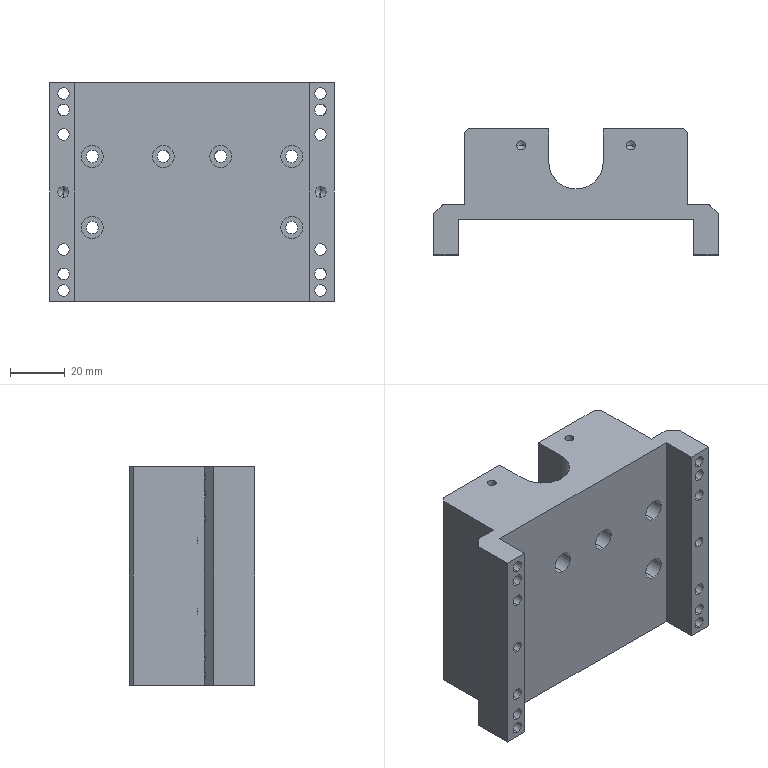Part | STEP file | X-axis lead screw slide - COMPANY_A version | 1 solid | 172 faces | box 104 x 46 x 80 mm | volume 190847 mm3 | cylinder 72 | plane 62 | cone 20 | spline 18 | commonest cylinder face diameters 4.2 x32 4.5 x12 8 x12 2.5 x4 3.3 x4 4 x4